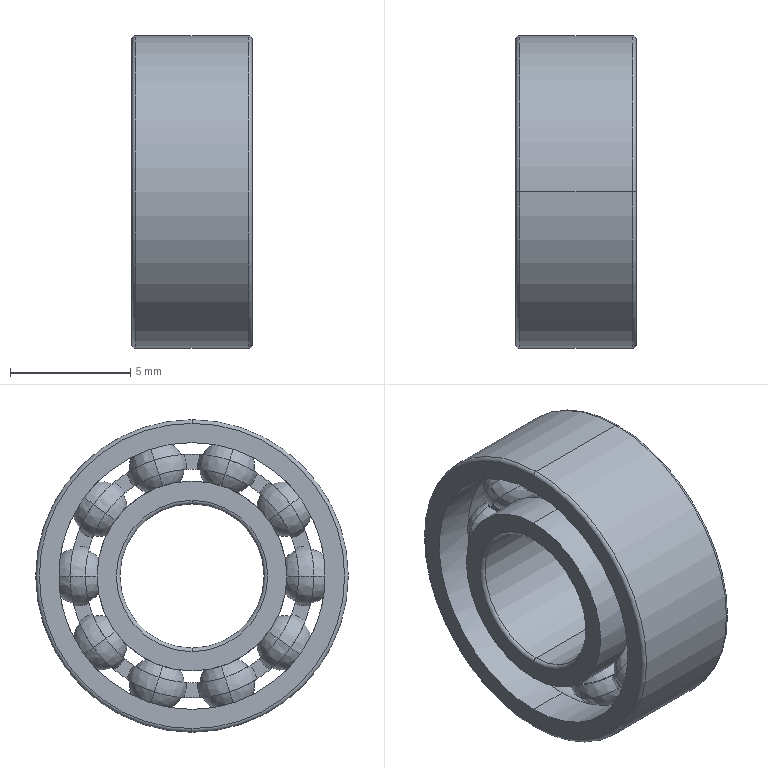Part | SolidWorks | features Revolution 5, CirPattern 2, RevCut 2 | 1 solid | 161 faces | box 5 x 13 x 13 mm | volume 330.95 mm3 | sphere 80 | torus 41 | plane 24 | cylinder 16 | commonest cylinder face diameters 7.9 x4 11.1 x4 6 x2 8.867 x2 10.132 x2 13 x2